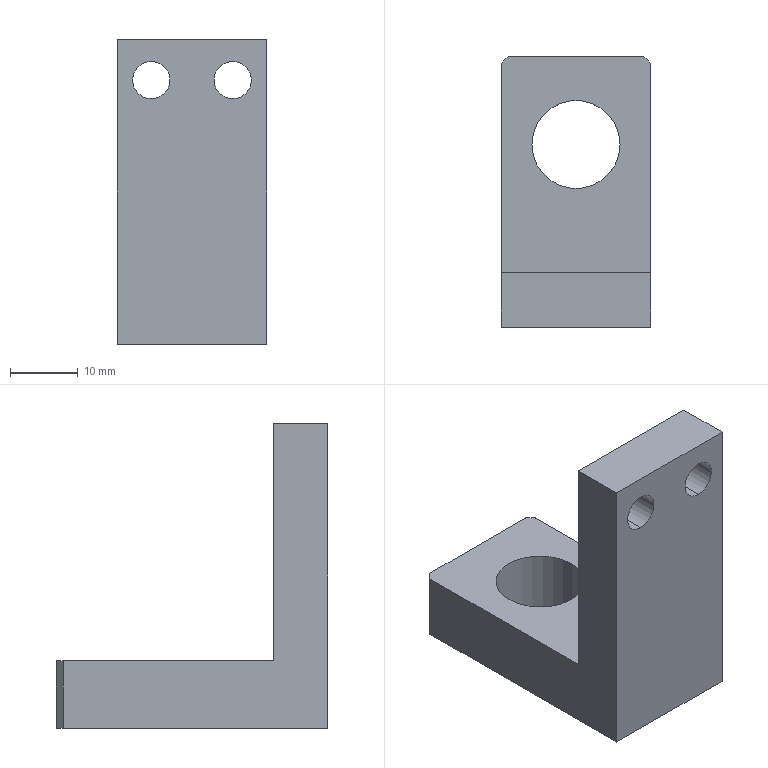Part | SolidWorks | features BaseBody 1, ICE 1, MoveFace 1 | 1 solid | 16 faces | box 22 x 40 x 45 mm | volume 13243 mm3 | plane 10 | cylinder 6 | commonest cylinder face diameters 5.5 x4 13 x2
STEP:
#1=CARTESIAN_POINT('',(6.5,7.,-13.));
#2=VERTEX_POINT('',#1);
#3=CARTESIAN_POINT('',(-6.5,7.,-13.));
#4=VERTEX_POINT('',#3);
#5=CARTESIAN_POINT('',(0.,7.,-13.));
#6=DIRECTION('',(0.,0.,-1.));
#7=DIRECTION('',(-1.,0.,0.));
#8=AXIS2_PLACEMENT_3D('',#5,#6,#7);
#9=CIRCLE('',#8,6.5);
#10=EDGE_CURVE('',#2,#4,#9,.T.);
#11=ORIENTED_EDGE('',*,*,#10,.F.);
#12=CARTESIAN_POINT('',(6.5,7.,-23.));
#13=VERTEX_POINT('',#12);
#14=CARTESIAN_POINT('',(6.5,7.,-13.));
#15=DIRECTION('',(0.,0.,-1.));
#16=VECTOR('',#15,1000.);
#17=LINE('',#14,#16);
#18=EDGE_CURVE('',#2,#13,#17,.T.);
#19=ORIENTED_EDGE('',*,*,#18,.T.);
#20=CARTESIAN_POINT('',(-6.5,7.,-23.));
#21=VERTEX_POINT('',#20);
#22=CARTESIAN_POINT('',(0.,7.,-23.));
#23=DIRECTION('',(0.,0.,-1.));
#24=DIRECTION('',(-1.,0.,0.));
#25=AXIS2_PLACEMENT_3D('',#22,#23,#24);
#26=CIRCLE('',#25,6.5);
#27=EDGE_CURVE('',#13,#21,#26,.T.);
#28=ORIENTED_EDGE('',*,*,#27,.T.);
#29=CARTESIAN_POINT('',(-6.5,7.,-13.));
#30=DIRECTION('',(0.,0.,-1.));
#31=VECTOR('',#30,1000.);
#32=LINE('',#29,#31);
#33=EDGE_CURVE('',#4,#21,#32,.T.);
#34=ORIENTED_EDGE('',*,*,#33,.F.);
#35=EDGE_LOOP('',(#11,#19,#28,#34));
#36=FACE_OUTER_BOUND('',#35,.T.);
#37=CARTESIAN_POINT('',(0.,7.,-13.));
#38=DIRECTION('',(0.,0.,-1.));
#39=DIRECTION('',(-1.,0.,0.));
#40=AXIS2_PLACEMENT_3D('',#37,#38,#39);
#41=CYLINDRICAL_SURFACE('',#40,6.5);
#42=ADVANCED_FACE('',(#36),#41,.F.);
#43=CARTESIAN_POINT('',(-6.,-20.,13.25));
#44=VERTEX_POINT('',#43);
#45=CARTESIAN_POINT('',(-6.,-12.,13.25));
#46=VERTEX_POINT('',#45);
#47=CARTESIAN_POINT('',(-6.,-20.,13.25));
#48=DIRECTION('',(0.,1.,0.));
#49=VECTOR('',#48,1000.);
#50=LINE('',#47,#49);
#51=EDGE_CURVE('',#44,#46,#50,.T.);
#52=ORIENTED_EDGE('',*,*,#51,.F.);
#53=CARTESIAN_POINT('',(-6.,-20.,18.75));
#54=VERTEX_POINT('',#53);
#55=CARTESIAN_POINT('',(-6.,-20.,16.));
#56=DIRECTION('',(0.,1.,0.));
#57=DIRECTION('',(0.,0.,1.));
#58=AXIS2_PLACEMENT_3D('',#55,#56,#57);
#59=CIRCLE('',#58,2.75);
#60=EDGE_CURVE('',#54,#44,#59,.T.);
#61=ORIENTED_EDGE('',*,*,#60,.F.);
#62=CARTESIAN_POINT('',(-6.,-12.,18.75));
#63=VERTEX_POINT('',#62);
#64=CARTESIAN_POINT('',(-6.,-20.,18.75));
#65=DIRECTION('',(0.,1.,0.));
#66=VECTOR('',#65,1000.);
#67=LINE('',#64,#66);
#68=EDGE_CURVE('',#54,#63,#67,.T.);
#69=ORIENTED_EDGE('',*,*,#68,.T.);
#70=CARTESIAN_POINT('',(-6.,-12.,16.));
#71=DIRECTION('',(0.,1.,0.));
#72=DIRECTION('',(0.,0.,1.));
#73=AXIS2_PLACEMENT_3D('',#70,#71,#72);
#74=CIRCLE('',#73,2.75);
#75=EDGE_CURVE('',#63,#46,#74,.T.);
#76=ORIENTED_EDGE('',*,*,#75,.T.);
#77=EDGE_LOOP('',(#52,#61,#69,#76));
#78=FACE_OUTER_BOUND('',#77,.T.);
#79=CARTESIAN_POINT('',(-6.,-20.,16.));
#80=DIRECTION('',(0.,1.,0.));
#81=DIRECTION('',(0.,0.,1.));
#82=AXIS2_PLACEMENT_3D('',#79,#80,#81);
#83=CYLINDRICAL_SURFACE('',#82,2.75);
#84=ADVANCED_FACE('',(#78),#83,.F.);
#85=CARTESIAN_POINT('',(6.,-20.,13.25));
#86=VERTEX_POINT('',#85);
#87=CARTESIAN_POINT('',(6.,-12.,13.25));
#88=VERTEX_POINT('',#87);
#89=CARTESIAN_POINT('',(6.,-20.,13.25));
#90=DIRECTION('',(0.,1.,0.));
#91=VECTOR('',#90,1000.);
#92=LINE('',#89,#91);
#93=EDGE_CURVE('',#86,#88,#92,.T.);
#94=ORIENTED_EDGE('',*,*,#93,.F.);
#95=CARTESIAN_POINT('',(6.,-20.,18.75));
#96=VERTEX_POINT('',#95);
#97=CARTESIAN_POINT('',(6.,-20.,16.));
#98=DIRECTION('',(0.,1.,0.));
#99=DIRECTION('',(0.,0.,1.));
#100=AXIS2_PLACEMENT_3D('',#97,#98,#99);
#101=CIRCLE('',#100,2.75);
#102=EDGE_CURVE('',#96,#86,#101,.T.);
#103=ORIENTED_EDGE('',*,*,#102,.F.);
#104=CARTESIAN_POINT('',(6.,-12.,18.75));
#105=VERTEX_POINT('',#104);
#106=CARTESIAN_POINT('',(6.,-20.,18.75));
#107=DIRECTION('',(0.,1.,0.));
#108=VECTOR('',#107,1000.);
#109=LINE('',#106,#108);
#110=EDGE_CURVE('',#96,#105,#109,.T.);
#111=ORIENTED_EDGE('',*,*,#110,.T.);
#112=CARTESIAN_POINT('',(6.,-12.,16.));
#113=DIRECTION('',(0.,1.,0.));
#114=DIRECTION('',(0.,0.,1.));
#115=AXIS2_PLACEMENT_3D('',#112,#113,#114);
#116=CIRCLE('',#115,2.75);
#117=EDGE_CURVE('',#105,#88,#116,.T.);
#118=ORIENTED_EDGE('',*,*,#117,.T.);
#119=EDGE_LOOP('',(#94,#103,#111,#118));
#120=FACE_OUTER_BOUND('',#119,.T.);
#121=CARTESIAN_POINT('',(6.,-20.,16.));
#122=DIRECTION('',(0.,1.,0.));
#123=DIRECTION('',(0.,0.,1.));
#124=AXIS2_PLACEMENT_3D('',#121,#122,#123);
#125=CYLINDRICAL_SURFACE('',#124,2.75);
#126=ADVANCED_FACE('',(#120),#125,.F.);
#127=CARTESIAN_POINT('',(-11.,-12.,22.));
#128=VERTEX_POINT('',#127);
#129=CARTESIAN_POINT('',(-11.,-20.,22.));
#130=VERTEX_POINT('',#129);
#131=CARTESIAN_POINT('',(-11.,-20.,22.));
#132=DIRECTION('',(0.,-1.,0.));
#133=VECTOR('',#132,1000.);
#134=LINE('',#131,#133);
#135=EDGE_CURVE('',#128,#130,#134,.T.);
#136=ORIENTED_EDGE('',*,*,#135,.T.);
#137=CARTESIAN_POINT('',(11.,-20.,22.));
#138=VERTEX_POINT('',#137);
#139=CARTESIAN_POINT('',(-11.,-20.,22.));
#140=DIRECTION('',(1.,0.,0.));
#141=VECTOR('',#140,1000.);
#142=LINE('',#139,#141);
#143=EDGE_CURVE('',#130,#138,#142,.T.);
#144=ORIENTED_EDGE('',*,*,#143,.T.);
#145=CARTESIAN_POINT('',(11.,-12.,22.));
#146=VERTEX_POINT('',#145);
#147=CARTESIAN_POINT('',(11.,-20.,22.));
#148=DIRECTION('',(0.,1.,0.));
#149=VECTOR('',#148,1000.);
#150=LINE('',#147,#149);
#151=EDGE_CURVE('',#138,#146,#150,.T.);
#152=ORIENTED_EDGE('',*,*,#151,.T.);
#153=CARTESIAN_POINT('',(-11.,-12.,22.));
#154=DIRECTION('',(-1.,0.,0.));
#155=VECTOR('',#154,1000.);
#156=LINE('',#153,#155);
#157=EDGE_CURVE('',#146,#128,#156,.T.);
#158=ORIENTED_EDGE('',*,*,#157,.T.);
#159=EDGE_LOOP('',(#136,#144,#152,#158));
#160=FACE_OUTER_BOUND('',#159,.T.);
#161=CARTESIAN_POINT('',(0.,0.,22.));
#162=DIRECTION('',(0.,0.,-1.));
#163=DIRECTION('',(0.,-1.,0.));
#164=AXIS2_PLACEMENT_3D('',#161,#162,#163);
#165=PLANE('',#164);
#166=ADVANCED_FACE('',(#160),#165,.F.);
#167=ORIENTED_EDGE('',*,*,#117,.F.);
#168=CARTESIAN_POINT('',(6.,-12.,16.));
#169=DIRECTION('',(0.,1.,0.));
#170=DIRECTION('',(0.,0.,1.));
#171=AXIS2_PLACEMENT_3D('',#168,#169,#170);
#172=CIRCLE('',#171,2.75);
#173=EDGE_CURVE('',#88,#105,#172,.T.);
#174=ORIENTED_EDGE('',*,*,#173,.F.);
#175=EDGE_LOOP('',(#167,#174));
#176=FACE_BOUND('',#175,.T.);
#177=ORIENTED_EDGE('',*,*,#75,.F.);
#178=CARTESIAN_POINT('',(-6.,-12.,16.));
#179=DIRECTION('',(0.,1.,0.));
#180=DIRECTION('',(0.,0.,1.));
#181=AXIS2_PLACEMENT_3D('',#178,#179,#180);
#182=CIRCLE('',#181,2.75);
#183=EDGE_CURVE('',#46,#63,#182,.T.);
#184=ORIENTED_EDGE('',*,*,#183,.F.);
#185=EDGE_LOOP('',(#177,#184));
#186=FACE_BOUND('',#185,.T.);
#187=CARTESIAN_POINT('',(11.,-12.,-13.));
#188=VERTEX_POINT('',#187);
#189=CARTESIAN_POINT('',(-11.,-12.,-13.));
#190=VERTEX_POINT('',#189);
#191=CARTESIAN_POINT('',(-11.,-12.,-13.));
#192=DIRECTION('',(-1.,0.,0.));
#193=VECTOR('',#192,1000.);
#194=LINE('',#191,#193);
#195=EDGE_CURVE('',#188,#190,#194,.T.);
#196=ORIENTED_EDGE('',*,*,#195,.T.);
#197=CARTESIAN_POINT('',(-11.,-12.,22.));
#198=DIRECTION('',(0.,0.,-1.));
#199=VECTOR('',#198,1000.);
#200=LINE('',#197,#199);
#201=EDGE_CURVE('',#128,#190,#200,.T.);
#202=ORIENTED_EDGE('',*,*,#201,.F.);
#203=ORIENTED_EDGE('',*,*,#157,.F.);
#204=CARTESIAN_POINT('',(11.,-12.,22.));
#205=DIRECTION('',(0.,0.,-1.));
#206=VECTOR('',#205,1000.);
#207=LINE('',#204,#206);
#208=EDGE_CURVE('',#146,#188,#207,.T.);
#209=ORIENTED_EDGE('',*,*,#208,.T.);
#210=EDGE_LOOP('',(#196,#202,#203,#209));
#211=FACE_OUTER_BOUND('',#210,.T.);
#212=CARTESIAN_POINT('',(-11.,-12.,22.));
#213=DIRECTION('',(0.,-1.,0.));
#214=DIRECTION('',(0.,0.,-1.));
#215=AXIS2_PLACEMENT_3D('',#212,#213,#214);
#216=PLANE('',#215);
#217=ADVANCED_FACE('',(#176,#186,#211),#216,.F.);
#218=CARTESIAN_POINT('',(-10.,20.,-13.));
#219=VERTEX_POINT('',#218);
#220=CARTESIAN_POINT('',(-11.,19.,-13.));
#221=VERTEX_POINT('',#220);
#222=CARTESIAN_POINT('',(-11.,19.,-13.));
#223=DIRECTION('',(-0.7071,-0.7071,0.));
#224=VECTOR('',#223,1000.);
#225=LINE('',#222,#224);
#226=EDGE_CURVE('',#219,#221,#225,.T.);
#227=ORIENTED_EDGE('',*,*,#226,.F.);
#228=CARTESIAN_POINT('',(-10.,20.,-23.));
#229=VERTEX_POINT('',#228);
#230=CARTESIAN_POINT('',(-10.,20.,10.));
#231=DIRECTION('',(0.,0.,1.));
#232=VECTOR('',#231,1000.);
#233=LINE('',#230,#232);
#234=EDGE_CURVE('',#229,#219,#233,.T.);
#235=ORIENTED_EDGE('',*,*,#234,.F.);
#236=CARTESIAN_POINT('',(-11.,19.,-23.));
#237=VERTEX_POINT('',#236);
#238=CARTESIAN_POINT('',(-15.,15.,-23.));
#239=DIRECTION('',(0.7071,0.7071,0.));
#240=VECTOR('',#239,1000.);
#241=LINE('',#238,#240);
#242=EDGE_CURVE('',#237,#229,#241,.T.);
#243=ORIENTED_EDGE('',*,*,#242,.F.);
#244=CARTESIAN_POINT('',(-11.,19.,10.));
#245=DIRECTION('',(0.,0.,-1.));
#246=VECTOR('',#245,1000.);
#247=LINE('',#244,#246);
#248=EDGE_CURVE('',#221,#237,#247,.T.);
#249=ORIENTED_EDGE('',*,*,#248,.F.);
#250=EDGE_LOOP('',(#227,#235,#243,#249));
#251=FACE_OUTER_BOUND('',#250,.T.);
#252=CARTESIAN_POINT('',(-11.,19.,10.));
#253=DIRECTION('',(0.7071,-0.7071,0.));
#254=DIRECTION('',(0.,0.,-1.));
#255=AXIS2_PLACEMENT_3D('',#252,#253,#254);
#256=PLANE('',#255);
#257=ADVANCED_FACE('',(#251),#256,.F.);
#258=CARTESIAN_POINT('',(11.,19.,-13.));
#259=VERTEX_POINT('',#258);
#260=CARTESIAN_POINT('',(10.,20.,-13.));
#261=VERTEX_POINT('',#260);
#262=CARTESIAN_POINT('',(10.,20.,-13.));
#263=DIRECTION('',(-0.7071,0.7071,0.));
#264=VECTOR('',#263,1000.);
#265=LINE('',#262,#264);
#266=EDGE_CURVE('',#259,#261,#265,.T.);
#267=ORIENTED_EDGE('',*,*,#266,.F.);
#268=CARTESIAN_POINT('',(11.,19.,-23.));
#269=VERTEX_POINT('',#268);
#270=CARTESIAN_POINT('',(11.,19.,10.));
#271=DIRECTION('',(0.,0.,1.));
#272=VECTOR('',#271,1000.);
#273=LINE('',#270,#272);
#274=EDGE_CURVE('',#269,#259,#273,.T.);
#275=ORIENTED_EDGE('',*,*,#274,.F.);
#276=CARTESIAN_POINT('',(10.,20.,-23.));
#277=VERTEX_POINT('',#276);
#278=CARTESIAN_POINT('',(15.,15.,-23.));
#279=DIRECTION('',(0.7071,-0.7071,0.));
#280=VECTOR('',#279,1000.);
#281=LINE('',#278,#280);
#282=EDGE_CURVE('',#277,#269,#281,.T.);
#283=ORIENTED_EDGE('',*,*,#282,.F.);
#284=CARTESIAN_POINT('',(10.,20.,10.));
#285=DIRECTION('',(0.,0.,-1.));
#286=VECTOR('',#285,1000.);
#287=LINE('',#284,#286);
#288=EDGE_CURVE('',#261,#277,#287,.T.);
#289=ORIENTED_EDGE('',*,*,#288,.F.);
#290=EDGE_LOOP('',(#267,#275,#283,#289));
#291=FACE_OUTER_BOUND('',#290,.T.);
#292=CARTESIAN_POINT('',(10.,20.,10.));
#293=DIRECTION('',(-0.7071,-0.7071,0.));
#294=DIRECTION('',(-0.7071,0.7071,0.));
#295=AXIS2_PLACEMENT_3D('',#292,#293,#294);
#296=PLANE('',#295);
#297=ADVANCED_FACE('',(#291),#296,.F.);
#298=CARTESIAN_POINT('',(-11.,20.,-23.));
#299=DIRECTION('',(-1.,0.,0.));
#300=VECTOR('',#299,1000.);
#301=LINE('',#298,#300);
#302=EDGE_CURVE('',#277,#229,#301,.T.);
#303=ORIENTED_EDGE('',*,*,#302,.F.);
#304=ORIENTED_EDGE('',*,*,#282,.T.);
#305=CARTESIAN_POINT('',(11.,-20.,-23.));
#306=VERTEX_POINT('',#305);
#307=CARTESIAN_POINT('',(11.,-20.,-23.));
#308=DIRECTION('',(0.,1.,0.));
#309=VECTOR('',#308,1000.);
#310=LINE('',#307,#309);
#311=EDGE_CURVE('',#306,#269,#310,.T.);
#312=ORIENTED_EDGE('',*,*,#311,.F.);
#313=CARTESIAN_POINT('',(-11.,-20.,-23.));
#314=VERTEX_POINT('',#313);
#315=CARTESIAN_POINT('',(-11.,-20.,-23.));
#316=DIRECTION('',(1.,0.,0.));
#317=VECTOR('',#316,1000.);
#318=LINE('',#315,#317);
#319=EDGE_CURVE('',#314,#306,#318,.T.);
#320=ORIENTED_EDGE('',*,*,#319,.F.);
#321=CARTESIAN_POINT('',(-11.,-20.,-23.));
#322=DIRECTION('',(0.,-1.,0.));
#323=VECTOR('',#322,1000.);
#324=LINE('',#321,#323);
#325=EDGE_CURVE('',#237,#314,#324,.T.);
#326=ORIENTED_EDGE('',*,*,#325,.F.);
#327=ORIENTED_EDGE('',*,*,#242,.T.);
#328=EDGE_LOOP('',(#303,#304,#312,#320,#326,#327));
#329=FACE_OUTER_BOUND('',#328,.T.);
#330=CARTESIAN_POINT('',(0.,7.,-23.));
#331=DIRECTION('',(0.,0.,-1.));
#332=DIRECTION('',(-1.,0.,0.));
#333=AXIS2_PLACEMENT_3D('',#330,#331,#332);
#334=CIRCLE('',#333,6.5);
#335=EDGE_CURVE('',#21,#13,#334,.T.);
#336=ORIENTED_EDGE('',*,*,#335,.F.);
#337=ORIENTED_EDGE('',*,*,#27,.F.);
#338=EDGE_LOOP('',(#336,#337));
#339=FACE_BOUND('',#338,.T.);
#340=CARTESIAN_POINT('',(0.,0.,-23.));
#341=DIRECTION('',(0.,0.,-1.));
#342=DIRECTION('',(0.,-1.,0.));
#343=AXIS2_PLACEMENT_3D('',#340,#341,#342);
#344=PLANE('',#343);
#345=ADVANCED_FACE('',(#329,#339),#344,.T.);
#346=ORIENTED_EDGE('',*,*,#102,.T.);
#347=CARTESIAN_POINT('',(6.,-20.,16.));
#348=DIRECTION('',(0.,1.,0.));
#349=DIRECTION('',(0.,0.,1.));
#350=AXIS2_PLACEMENT_3D('',#347,#348,#349);
#351=CIRCLE('',#350,2.75);
#352=EDGE_CURVE('',#86,#96,#351,.T.);
#353=ORIENTED_EDGE('',*,*,#352,.T.);
#354=EDGE_LOOP('',(#346,#353));
#355=FACE_BOUND('',#354,.T.);
#356=ORIENTED_EDGE('',*,*,#60,.T.);
#357=CARTESIAN_POINT('',(-6.,-20.,16.));
#358=DIRECTION('',(0.,1.,0.));
#359=DIRECTION('',(0.,0.,1.));
#360=AXIS2_PLACEMENT_3D('',#357,#358,#359);
#361=CIRCLE('',#360,2.75);
#362=EDGE_CURVE('',#44,#54,#361,.T.);
#363=ORIENTED_EDGE('',*,*,#362,.T.);
#364=EDGE_LOOP('',(#356,#363));
#365=FACE_BOUND('',#364,.T.);
#366=ORIENTED_EDGE('',*,*,#319,.T.);
#367=CARTESIAN_POINT('',(11.,-20.,10.));
#368=DIRECTION('',(0.,0.,-1.));
#369=VECTOR('',#368,1000.);
#370=LINE('',#367,#369);
#371=EDGE_CURVE('',#138,#306,#370,.T.);
#372=ORIENTED_EDGE('',*,*,#371,.F.);
#373=ORIENTED_EDGE('',*,*,#143,.F.);
#374=CARTESIAN_POINT('',(-11.,-20.,10.));
#375=DIRECTION('',(0.,0.,-1.));
#376=VECTOR('',#375,1000.);
#377=LINE('',#374,#376);
#378=EDGE_CURVE('',#130,#314,#377,.T.);
#379=ORIENTED_EDGE('',*,*,#378,.T.);
#380=EDGE_LOOP('',(#366,#372,#373,#379));
#381=FACE_OUTER_BOUND('',#380,.T.);
#382=CARTESIAN_POINT('',(-11.,-20.,10.));
#383=DIRECTION('',(0.,1.,0.));
#384=DIRECTION('',(1.,0.,0.));
#385=AXIS2_PLACEMENT_3D('',#382,#383,#384);
#386=PLANE('',#385);
#387=ADVANCED_FACE('',(#355,#365,#381),#386,.F.);
#388=CARTESIAN_POINT('',(-11.,-20.,-13.));
#389=DIRECTION('',(0.,-1.,0.));
#390=VECTOR('',#389,1000.);
#391=LINE('',#388,#390);
#392=EDGE_CURVE('',#221,#190,#391,.T.);
#393=ORIENTED_EDGE('',*,*,#392,.F.);
#394=ORIENTED_EDGE('',*,*,#248,.T.);
#395=ORIENTED_EDGE('',*,*,#325,.T.);
#396=ORIENTED_EDGE('',*,*,#378,.F.);
#397=ORIENTED_EDGE('',*,*,#135,.F.);
#398=ORIENTED_EDGE('',*,*,#201,.T.);
#399=EDGE_LOOP('',(#393,#394,#395,#396,#397,#398));
#400=FACE_OUTER_BOUND('',#399,.T.);
#401=CARTESIAN_POINT('',(-11.,-20.,10.));
#402=DIRECTION('',(1.,0.,0.));
#403=DIRECTION('',(0.,1.,0.));
#404=AXIS2_PLACEMENT_3D('',#401,#402,#403);
#405=PLANE('',#404);
#406=ADVANCED_FACE('',(#400),#405,.F.);
#407=CARTESIAN_POINT('',(-11.,20.,-13.));
#408=DIRECTION('',(-1.,0.,0.));
#409=VECTOR('',#408,1000.);
#410=LINE('',#407,#409);
#411=EDGE_CURVE('',#261,#219,#410,.T.);
#412=ORIENTED_EDGE('',*,*,#411,.F.);
#413=ORIENTED_EDGE('',*,*,#288,.T.);
#414=ORIENTED_EDGE('',*,*,#302,.T.);
#415=ORIENTED_EDGE('',*,*,#234,.T.);
#416=EDGE_LOOP('',(#412,#413,#414,#415));
#417=FACE_OUTER_BOUND('',#416,.T.);
#418=CARTESIAN_POINT('',(-11.,20.,10.));
#419=DIRECTION('',(0.,-1.,0.));
#420=DIRECTION('',(0.,0.,-1.));
#421=AXIS2_PLACEMENT_3D('',#418,#419,#420);
#422=PLANE('',#421);
#423=ADVANCED_FACE('',(#417),#422,.F.);
#424=ORIENTED_EDGE('',*,*,#311,.T.);
#425=ORIENTED_EDGE('',*,*,#274,.T.);
#426=CARTESIAN_POINT('',(11.,-20.,-13.));
#427=DIRECTION('',(0.,1.,0.));
#428=VECTOR('',#427,1000.);
#429=LINE('',#426,#428);
#430=EDGE_CURVE('',#188,#259,#429,.T.);
#431=ORIENTED_EDGE('',*,*,#430,.F.);
#432=ORIENTED_EDGE('',*,*,#208,.F.);
#433=ORIENTED_EDGE('',*,*,#151,.F.);
#434=ORIENTED_EDGE('',*,*,#371,.T.);
#435=EDGE_LOOP('',(#424,#425,#431,#432,#433,#434));
#436=FACE_OUTER_BOUND('',#435,.T.);
#437=CARTESIAN_POINT('',(11.,-20.,10.));
#438=DIRECTION('',(-1.,0.,0.));
#439=DIRECTION('',(0.,0.,1.));
#440=AXIS2_PLACEMENT_3D('',#437,#438,#439);
#441=PLANE('',#440);
#442=ADVANCED_FACE('',(#436),#441,.F.);
#443=ORIENTED_EDGE('',*,*,#195,.F.);
#444=ORIENTED_EDGE('',*,*,#430,.T.);
#445=ORIENTED_EDGE('',*,*,#266,.T.);
#446=ORIENTED_EDGE('',*,*,#411,.T.);
#447=ORIENTED_EDGE('',*,*,#226,.T.);
#448=ORIENTED_EDGE('',*,*,#392,.T.);
#449=EDGE_LOOP('',(#443,#444,#445,#446,#447,#448));
#450=FACE_OUTER_BOUND('',#449,.T.);
#451=CARTESIAN_POINT('',(0.,7.,-13.));
#452=DIRECTION('',(0.,0.,-1.));
#453=DIRECTION('',(-1.,0.,0.));
#454=AXIS2_PLACEMENT_3D('',#451,#452,#453);
#455=CIRCLE('',#454,6.5);
#456=EDGE_CURVE('',#4,#2,#455,.T.);
#457=ORIENTED_EDGE('',*,*,#456,.T.);
#458=ORIENTED_EDGE('',*,*,#10,.T.);
#459=EDGE_LOOP('',(#457,#458));
#460=FACE_BOUND('',#459,.T.);
#461=CARTESIAN_POINT('',(0.,0.,-13.));
#462=DIRECTION('',(0.,0.,-1.));
#463=DIRECTION('',(0.,-1.,0.));
#464=AXIS2_PLACEMENT_3D('',#461,#462,#463);
#465=PLANE('',#464);
#466=ADVANCED_FACE('',(#450,#460),#465,.F.);
#467=ORIENTED_EDGE('',*,*,#352,.F.);
#468=ORIENTED_EDGE('',*,*,#93,.T.);
#469=ORIENTED_EDGE('',*,*,#173,.T.);
#470=ORIENTED_EDGE('',*,*,#110,.F.);
#471=EDGE_LOOP('',(#467,#468,#469,#470));
#472=FACE_OUTER_BOUND('',#471,.T.);
#473=CARTESIAN_POINT('',(6.,-20.,16.));
#474=DIRECTION('',(0.,1.,0.));
#475=DIRECTION('',(0.,0.,1.));
#476=AXIS2_PLACEMENT_3D('',#473,#474,#475);
#477=CYLINDRICAL_SURFACE('',#476,2.75);
#478=ADVANCED_FACE('',(#472),#477,.F.);
#479=ORIENTED_EDGE('',*,*,#362,.F.);
#480=ORIENTED_EDGE('',*,*,#51,.T.);
#481=ORIENTED_EDGE('',*,*,#183,.T.);
#482=ORIENTED_EDGE('',*,*,#68,.F.);
#483=EDGE_LOOP('',(#479,#480,#481,#482));
#484=FACE_OUTER_BOUND('',#483,.T.);
#485=CARTESIAN_POINT('',(-6.,-20.,16.));
#486=DIRECTION('',(0.,1.,0.));
#487=DIRECTION('',(0.,0.,1.));
#488=AXIS2_PLACEMENT_3D('',#485,#486,#487);
#489=CYLINDRICAL_SURFACE('',#488,2.75);
#490=ADVANCED_FACE('',(#484),#489,.F.);
#491=ORIENTED_EDGE('',*,*,#18,.F.);
#492=ORIENTED_EDGE('',*,*,#456,.F.);
#493=ORIENTED_EDGE('',*,*,#33,.T.);
#494=ORIENTED_EDGE('',*,*,#335,.T.);
#495=EDGE_LOOP('',(#491,#492,#493,#494));
#496=FACE_OUTER_BOUND('',#495,.T.);
#497=CARTESIAN_POINT('',(0.,7.,-13.));
#498=DIRECTION('',(0.,0.,-1.));
#499=DIRECTION('',(-1.,0.,0.));
#500=AXIS2_PLACEMENT_3D('',#497,#498,#499);
#501=CYLINDRICAL_SURFACE('',#500,6.5);
#502=ADVANCED_FACE('',(#496),#501,.F.);
#503=CLOSED_SHELL('',(#42,#84,#126,#166,#217,#257,#297,#345,#387,#406,#423,#442,#466,#478,#490,#502));
#504=MANIFOLD_SOLID_BREP('',#503);
#505=CARTESIAN_POINT('',(0.,0.,0.));
#506=DIRECTION('',(0.,0.,1.));
#507=DIRECTION('',(1.,0.,0.));
#508=AXIS2_PLACEMENT_3D('',#505,#506,#507);
#509=(LENGTH_UNIT()NAMED_UNIT(*)SI_UNIT(.MILLI.,.METRE.));
#510=UNCERTAINTY_MEASURE_WITH_UNIT(LENGTH_MEASURE(0.00001),#509,'','');
#511=(NAMED_UNIT(*)PLANE_ANGLE_UNIT()SI_UNIT($,.RADIAN.));
#512=(NAMED_UNIT(*)SI_UNIT($,.STERADIAN.)SOLID_ANGLE_UNIT());
#513=(GEOMETRIC_REPRESENTATION_CONTEXT(3)GLOBAL_UNCERTAINTY_ASSIGNED_CONTEXT((#510))GLOBAL_UNIT_ASSIGNED_CONTEXT((#509,#511,#512))REPRESENTATION_CONTEXT('',''));
#514=ADVANCED_BREP_SHAPE_REPRESENTATION('',(#504,#508),#513);